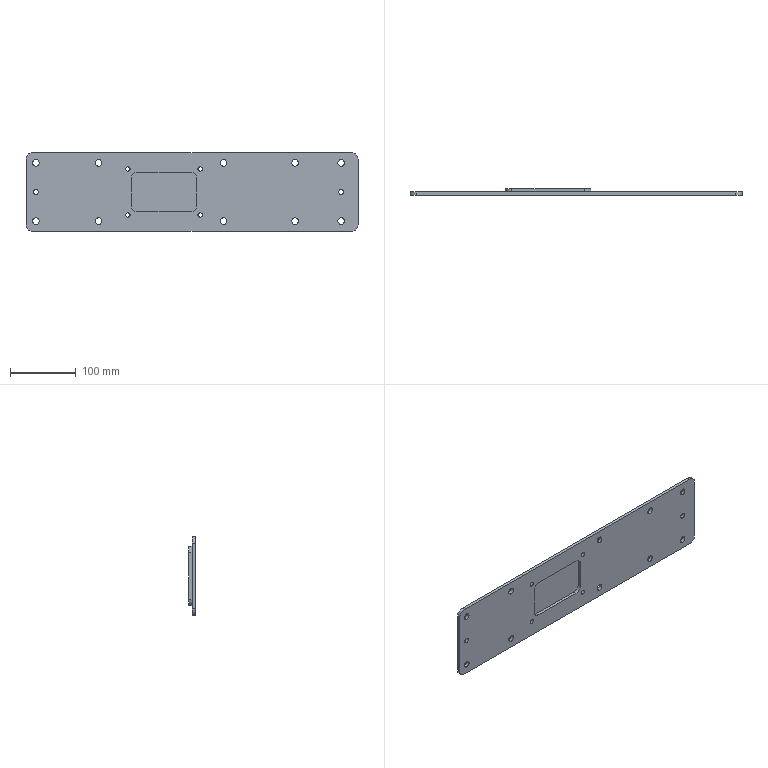Part | SolidWorks | features Fillet 2, ICE 2, Extrusion 1, HoleWzd 1 | 2 solids | 68 faces | box 505 x 10 x 120 mm | volume 325188 mm3 | cylinder 52 | plane 16 | commonest cylinder face diameters 10 x20 6.8 x16 20 x12 8 x4